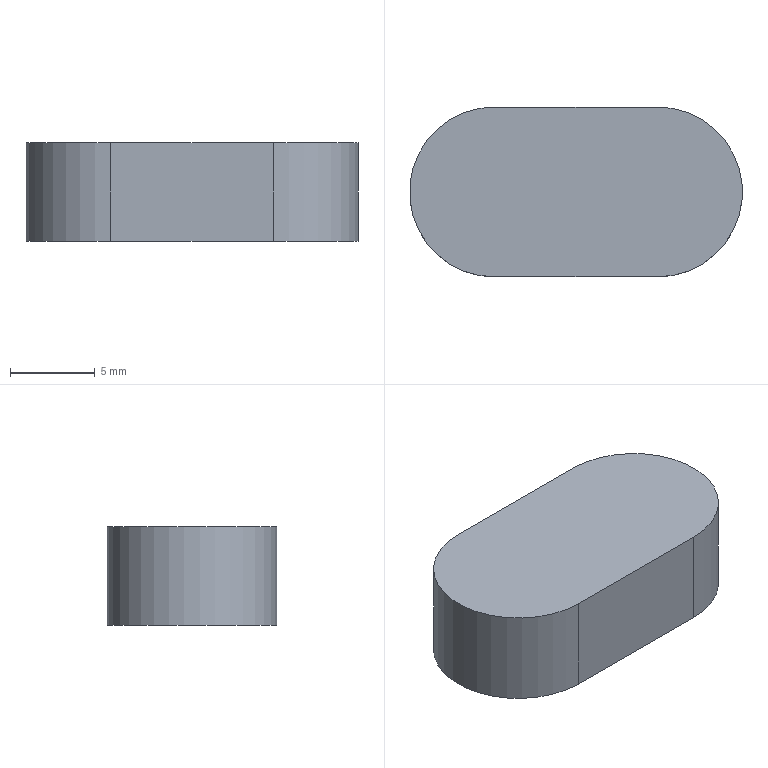Part | NX | features DATUM_CSYS 2, EXTRUDE 1, SKETCH 1 | 1 solid | 6 faces | box 19.6 x 10 x 5.8 mm | volume 1012 mm3 | plane 4 | cylinder 2 | commonest cylinder face diameters 10 x2
STEP:
#1=CARTESIAN_POINT('',(-4.8,5.,0.));
#2=VERTEX_POINT('',#1);
#3=CARTESIAN_POINT('',(-4.8,-5.,0.));
#4=VERTEX_POINT('',#3);
#5=CARTESIAN_POINT('',(-4.8,0.,0.));
#6=DIRECTION('',(0.,0.,1.));
#7=DIRECTION('',(-1.,0.,0.));
#8=AXIS2_PLACEMENT_3D('',#5,#6,#7);
#9=CIRCLE('',#8,5.);
#10=EDGE_CURVE('',#2,#4,#9,.T.);
#11=ORIENTED_EDGE('',*,*,#10,.T.);
#12=CARTESIAN_POINT('',(-4.8,-5.,5.8));
#13=VERTEX_POINT('',#12);
#14=CARTESIAN_POINT('',(-4.8,-5.,5.8));
#15=DIRECTION('',(0.,0.,-1.));
#16=VECTOR('',#15,1000.);
#17=LINE('',#14,#16);
#18=EDGE_CURVE('',#13,#4,#17,.T.);
#19=ORIENTED_EDGE('',*,*,#18,.F.);
#20=CARTESIAN_POINT('',(-4.8,5.,5.8));
#21=VERTEX_POINT('',#20);
#22=CARTESIAN_POINT('',(-4.8,0.,5.8));
#23=DIRECTION('',(0.,0.,1.));
#24=DIRECTION('',(-1.,0.,0.));
#25=AXIS2_PLACEMENT_3D('',#22,#23,#24);
#26=CIRCLE('',#25,5.);
#27=EDGE_CURVE('',#21,#13,#26,.T.);
#28=ORIENTED_EDGE('',*,*,#27,.F.);
#29=CARTESIAN_POINT('',(-4.8,5.,5.8));
#30=DIRECTION('',(0.,0.,-1.));
#31=VECTOR('',#30,1000.);
#32=LINE('',#29,#31);
#33=EDGE_CURVE('',#21,#2,#32,.T.);
#34=ORIENTED_EDGE('',*,*,#33,.T.);
#35=EDGE_LOOP('',(#11,#19,#28,#34));
#36=FACE_BOUND('',#35,.T.);
#37=CARTESIAN_POINT('',(-4.8,0.,5.8));
#38=DIRECTION('',(0.,0.,-1.));
#39=DIRECTION('',(-1.,0.,0.));
#40=AXIS2_PLACEMENT_3D('',#37,#38,#39);
#41=CYLINDRICAL_SURFACE('',#40,5.);
#42=ADVANCED_FACE('',(#36),#41,.T.);
#43=CARTESIAN_POINT('',(4.8,-5.,0.));
#44=VERTEX_POINT('',#43);
#45=CARTESIAN_POINT('',(-4.8,-5.,0.));
#46=DIRECTION('',(1.,0.,0.));
#47=VECTOR('',#46,1000.);
#48=LINE('',#45,#47);
#49=EDGE_CURVE('',#4,#44,#48,.T.);
#50=ORIENTED_EDGE('',*,*,#49,.T.);
#51=CARTESIAN_POINT('',(4.8,-5.,5.8));
#52=VERTEX_POINT('',#51);
#53=CARTESIAN_POINT('',(4.8,-5.,5.8));
#54=DIRECTION('',(0.,0.,-1.));
#55=VECTOR('',#54,1000.);
#56=LINE('',#53,#55);
#57=EDGE_CURVE('',#52,#44,#56,.T.);
#58=ORIENTED_EDGE('',*,*,#57,.F.);
#59=CARTESIAN_POINT('',(-4.8,-5.,5.8));
#60=DIRECTION('',(1.,0.,0.));
#61=VECTOR('',#60,1000.);
#62=LINE('',#59,#61);
#63=EDGE_CURVE('',#13,#52,#62,.T.);
#64=ORIENTED_EDGE('',*,*,#63,.F.);
#65=ORIENTED_EDGE('',*,*,#18,.T.);
#66=EDGE_LOOP('',(#50,#58,#64,#65));
#67=FACE_BOUND('',#66,.T.);
#68=CARTESIAN_POINT('',(-4.8,-5.,5.8));
#69=DIRECTION('',(0.,1.,0.));
#70=DIRECTION('',(0.,0.,1.));
#71=AXIS2_PLACEMENT_3D('',#68,#69,#70);
#72=PLANE('',#71);
#73=ADVANCED_FACE('',(#67),#72,.F.);
#74=CARTESIAN_POINT('',(4.8,5.,0.));
#75=VERTEX_POINT('',#74);
#76=CARTESIAN_POINT('',(4.8,0.,0.));
#77=DIRECTION('',(0.,0.,1.));
#78=DIRECTION('',(1.,0.,0.));
#79=AXIS2_PLACEMENT_3D('',#76,#77,#78);
#80=CIRCLE('',#79,5.);
#81=EDGE_CURVE('',#44,#75,#80,.T.);
#82=ORIENTED_EDGE('',*,*,#81,.T.);
#83=CARTESIAN_POINT('',(4.8,5.,5.8));
#84=VERTEX_POINT('',#83);
#85=CARTESIAN_POINT('',(4.8,5.,5.8));
#86=DIRECTION('',(0.,0.,-1.));
#87=VECTOR('',#86,1000.);
#88=LINE('',#85,#87);
#89=EDGE_CURVE('',#84,#75,#88,.T.);
#90=ORIENTED_EDGE('',*,*,#89,.F.);
#91=CARTESIAN_POINT('',(4.8,0.,5.8));
#92=DIRECTION('',(0.,0.,1.));
#93=DIRECTION('',(1.,0.,0.));
#94=AXIS2_PLACEMENT_3D('',#91,#92,#93);
#95=CIRCLE('',#94,5.);
#96=EDGE_CURVE('',#52,#84,#95,.T.);
#97=ORIENTED_EDGE('',*,*,#96,.F.);
#98=ORIENTED_EDGE('',*,*,#57,.T.);
#99=EDGE_LOOP('',(#82,#90,#97,#98));
#100=FACE_BOUND('',#99,.T.);
#101=CARTESIAN_POINT('',(4.8,0.,5.8));
#102=DIRECTION('',(0.,0.,-1.));
#103=DIRECTION('',(-1.,0.,0.));
#104=AXIS2_PLACEMENT_3D('',#101,#102,#103);
#105=CYLINDRICAL_SURFACE('',#104,5.);
#106=ADVANCED_FACE('',(#100),#105,.T.);
#107=CARTESIAN_POINT('',(4.8,5.,0.));
#108=DIRECTION('',(-1.,0.,0.));
#109=VECTOR('',#108,1000.);
#110=LINE('',#107,#109);
#111=EDGE_CURVE('',#75,#2,#110,.T.);
#112=ORIENTED_EDGE('',*,*,#111,.T.);
#113=ORIENTED_EDGE('',*,*,#33,.F.);
#114=CARTESIAN_POINT('',(4.8,5.,5.8));
#115=DIRECTION('',(-1.,0.,0.));
#116=VECTOR('',#115,1000.);
#117=LINE('',#114,#116);
#118=EDGE_CURVE('',#84,#21,#117,.T.);
#119=ORIENTED_EDGE('',*,*,#118,.F.);
#120=ORIENTED_EDGE('',*,*,#89,.T.);
#121=EDGE_LOOP('',(#112,#113,#119,#120));
#122=FACE_BOUND('',#121,.T.);
#123=CARTESIAN_POINT('',(4.8,5.,5.8));
#124=DIRECTION('',(0.,-1.,0.));
#125=DIRECTION('',(0.,0.,-1.));
#126=AXIS2_PLACEMENT_3D('',#123,#124,#125);
#127=PLANE('',#126);
#128=ADVANCED_FACE('',(#122),#127,.F.);
#129=ORIENTED_EDGE('',*,*,#27,.T.);
#130=ORIENTED_EDGE('',*,*,#63,.T.);
#131=ORIENTED_EDGE('',*,*,#96,.T.);
#132=ORIENTED_EDGE('',*,*,#118,.T.);
#133=EDGE_LOOP('',(#129,#130,#131,#132));
#134=FACE_BOUND('',#133,.T.);
#135=CARTESIAN_POINT('',(-4.8,0.,5.8));
#136=DIRECTION('',(0.,0.,1.));
#137=DIRECTION('',(1.,0.,0.));
#138=AXIS2_PLACEMENT_3D('',#135,#136,#137);
#139=PLANE('',#138);
#140=ADVANCED_FACE('',(#134),#139,.T.);
#141=ORIENTED_EDGE('',*,*,#10,.F.);
#142=ORIENTED_EDGE('',*,*,#111,.F.);
#143=ORIENTED_EDGE('',*,*,#81,.F.);
#144=ORIENTED_EDGE('',*,*,#49,.F.);
#145=EDGE_LOOP('',(#141,#142,#143,#144));
#146=FACE_BOUND('',#145,.T.);
#147=CARTESIAN_POINT('',(-4.8,0.,0.));
#148=DIRECTION('',(0.,0.,1.));
#149=DIRECTION('',(1.,0.,0.));
#150=AXIS2_PLACEMENT_3D('',#147,#148,#149);
#151=PLANE('',#150);
#152=ADVANCED_FACE('',(#146),#151,.F.);
#153=CLOSED_SHELL('',(#42,#73,#106,#128,#140,#152));
#154=MANIFOLD_SOLID_BREP('',#153);
#155=(LENGTH_UNIT()NAMED_UNIT(*)SI_UNIT(.MILLI.,.METRE.));
#156=UNCERTAINTY_MEASURE_WITH_UNIT(LENGTH_MEASURE(0.00001),#155,'','');
#157=(NAMED_UNIT(*)PLANE_ANGLE_UNIT()SI_UNIT($,.RADIAN.));
#158=(NAMED_UNIT(*)SI_UNIT($,.STERADIAN.)SOLID_ANGLE_UNIT());
#159=(GEOMETRIC_REPRESENTATION_CONTEXT(3)GLOBAL_UNCERTAINTY_ASSIGNED_CONTEXT((#156))GLOBAL_UNIT_ASSIGNED_CONTEXT((#155,#157,#158))REPRESENTATION_CONTEXT('',''));
#160=ADVANCED_BREP_SHAPE_REPRESENTATION('',(#154),#159);